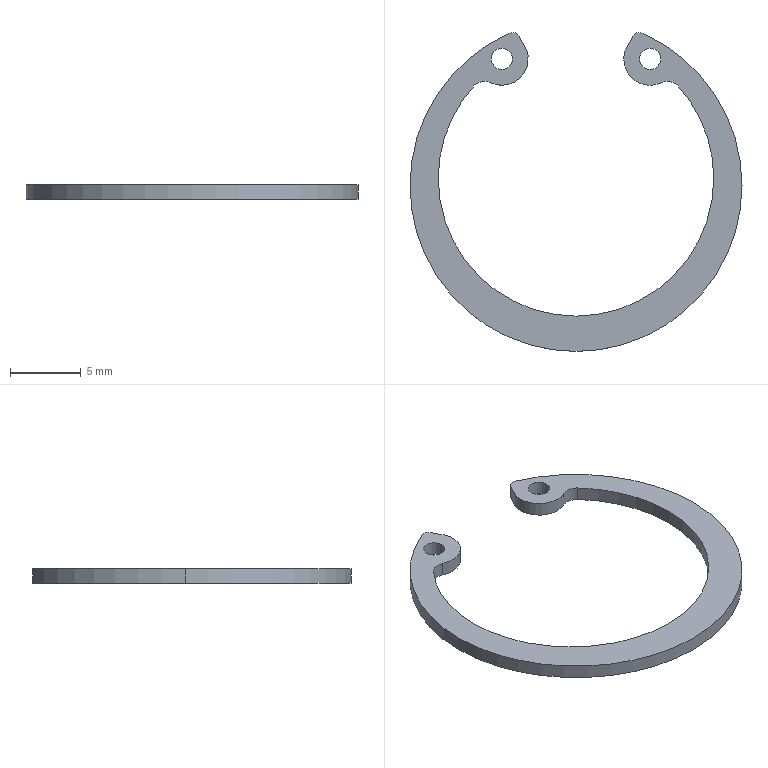Part | 1 solid | 21 faces | box 23.5 x 22.573 x 1 mm | volume 128.743 mm3 | cylinder 17 | plane 4 | commonest cylinder face diameters 1.5 x4 3.731 x3 19.5 x3 23.5 x3 1 x2 2 x2
STEP:
#1=CARTESIAN_POINT('',(4.5,8.954,1.));
#2=VERTEX_POINT('',#1);
#3=CARTESIAN_POINT('',(6.,8.954,1.));
#4=VERTEX_POINT('',#3);
#5=CARTESIAN_POINT('',(5.25,8.954,1.));
#6=DIRECTION('',(0.,0.,1.));
#7=DIRECTION('',(-1.,0.,0.));
#8=AXIS2_PLACEMENT_3D('',#5,#6,#7);
#9=CIRCLE('',#8,0.75);
#10=EDGE_CURVE('',#2,#4,#9,.T.);
#11=ORIENTED_EDGE('',*,*,#10,.T.);
#12=CARTESIAN_POINT('',(6.,8.954,0.));
#13=VERTEX_POINT('',#12);
#14=CARTESIAN_POINT('',(6.,8.954,1.));
#15=DIRECTION('',(0.,0.,-1.));
#16=VECTOR('',#15,1000.);
#17=LINE('',#14,#16);
#18=EDGE_CURVE('',#4,#13,#17,.T.);
#19=ORIENTED_EDGE('',*,*,#18,.T.);
#20=CARTESIAN_POINT('',(4.5,8.954,0.));
#21=VERTEX_POINT('',#20);
#22=CARTESIAN_POINT('',(5.25,8.954,0.));
#23=DIRECTION('',(0.,0.,1.));
#24=DIRECTION('',(-1.,0.,0.));
#25=AXIS2_PLACEMENT_3D('',#22,#23,#24);
#26=CIRCLE('',#25,0.75);
#27=EDGE_CURVE('',#21,#13,#26,.T.);
#28=ORIENTED_EDGE('',*,*,#27,.F.);
#29=CARTESIAN_POINT('',(4.5,8.954,1.));
#30=DIRECTION('',(0.,0.,-1.));
#31=VECTOR('',#30,1000.);
#32=LINE('',#29,#31);
#33=EDGE_CURVE('',#2,#21,#32,.T.);
#34=ORIENTED_EDGE('',*,*,#33,.F.);
#35=EDGE_LOOP('',(#11,#19,#28,#34));
#36=FACE_OUTER_BOUND('',#35,.T.);
#37=CARTESIAN_POINT('',(5.25,8.954,1.));
#38=DIRECTION('',(0.,0.,-1.));
#39=DIRECTION('',(-1.,0.,0.));
#40=AXIS2_PLACEMENT_3D('',#37,#38,#39);
#41=CYLINDRICAL_SURFACE('',#40,0.75);
#42=ADVANCED_FACE('',(#36),#41,.F.);
#43=CARTESIAN_POINT('',(-6.,8.954,1.));
#44=VERTEX_POINT('',#43);
#45=CARTESIAN_POINT('',(-4.5,8.954,1.));
#46=VERTEX_POINT('',#45);
#47=CARTESIAN_POINT('',(-5.25,8.954,1.));
#48=DIRECTION('',(0.,0.,1.));
#49=DIRECTION('',(1.,0.,0.));
#50=AXIS2_PLACEMENT_3D('',#47,#48,#49);
#51=CIRCLE('',#50,0.75);
#52=EDGE_CURVE('',#44,#46,#51,.T.);
#53=ORIENTED_EDGE('',*,*,#52,.T.);
#54=CARTESIAN_POINT('',(-4.5,8.954,0.));
#55=VERTEX_POINT('',#54);
#56=CARTESIAN_POINT('',(-4.5,8.954,1.));
#57=DIRECTION('',(0.,0.,-1.));
#58=VECTOR('',#57,1000.);
#59=LINE('',#56,#58);
#60=EDGE_CURVE('',#46,#55,#59,.T.);
#61=ORIENTED_EDGE('',*,*,#60,.T.);
#62=CARTESIAN_POINT('',(-6.,8.954,0.));
#63=VERTEX_POINT('',#62);
#64=CARTESIAN_POINT('',(-5.25,8.954,0.));
#65=DIRECTION('',(0.,0.,1.));
#66=DIRECTION('',(1.,0.,0.));
#67=AXIS2_PLACEMENT_3D('',#64,#65,#66);
#68=CIRCLE('',#67,0.75);
#69=EDGE_CURVE('',#63,#55,#68,.T.);
#70=ORIENTED_EDGE('',*,*,#69,.F.);
#71=CARTESIAN_POINT('',(-6.,8.954,1.));
#72=DIRECTION('',(0.,0.,-1.));
#73=VECTOR('',#72,1000.);
#74=LINE('',#71,#73);
#75=EDGE_CURVE('',#44,#63,#74,.T.);
#76=ORIENTED_EDGE('',*,*,#75,.F.);
#77=EDGE_LOOP('',(#53,#61,#70,#76));
#78=FACE_OUTER_BOUND('',#77,.T.);
#79=CARTESIAN_POINT('',(-5.25,8.954,1.));
#80=DIRECTION('',(0.,0.,-1.));
#81=DIRECTION('',(-1.,0.,0.));
#82=AXIS2_PLACEMENT_3D('',#79,#80,#81);
#83=CYLINDRICAL_SURFACE('',#82,0.75);
#84=ADVANCED_FACE('',(#78),#83,.F.);
#85=CARTESIAN_POINT('',(11.75,0.,1.));
#86=VERTEX_POINT('',#85);
#87=CARTESIAN_POINT('',(4.671,10.782,1.));
#88=VERTEX_POINT('',#87);
#89=CARTESIAN_POINT('',(0.,0.,1.));
#90=DIRECTION('',(0.,0.,1.));
#91=DIRECTION('',(1.,0.,0.));
#92=AXIS2_PLACEMENT_3D('',#89,#90,#91);
#93=CIRCLE('',#92,11.75);
#94=EDGE_CURVE('',#86,#88,#93,.T.);
#95=ORIENTED_EDGE('',*,*,#94,.F.);
#96=CARTESIAN_POINT('',(11.75,0.,0.));
#97=VERTEX_POINT('',#96);
#98=CARTESIAN_POINT('',(11.75,0.,1.));
#99=DIRECTION('',(0.,0.,-1.));
#100=VECTOR('',#99,1000.);
#101=LINE('',#98,#100);
#102=EDGE_CURVE('',#86,#97,#101,.T.);
#103=ORIENTED_EDGE('',*,*,#102,.T.);
#104=CARTESIAN_POINT('',(4.671,10.782,0.));
#105=VERTEX_POINT('',#104);
#106=CARTESIAN_POINT('',(0.,0.,0.));
#107=DIRECTION('',(0.,0.,1.));
#108=DIRECTION('',(1.,0.,0.));
#109=AXIS2_PLACEMENT_3D('',#106,#107,#108);
#110=CIRCLE('',#109,11.75);
#111=EDGE_CURVE('',#97,#105,#110,.T.);
#112=ORIENTED_EDGE('',*,*,#111,.T.);
#113=CARTESIAN_POINT('',(4.671,10.782,1.));
#114=DIRECTION('',(0.,0.,-1.));
#115=VECTOR('',#114,1000.);
#116=LINE('',#113,#115);
#117=EDGE_CURVE('',#88,#105,#116,.T.);
#118=ORIENTED_EDGE('',*,*,#117,.F.);
#119=EDGE_LOOP('',(#95,#103,#112,#118));
#120=FACE_OUTER_BOUND('',#119,.T.);
#121=CARTESIAN_POINT('',(0.,0.,1.));
#122=DIRECTION('',(0.,0.,-1.));
#123=DIRECTION('',(-1.,0.,0.));
#124=AXIS2_PLACEMENT_3D('',#121,#122,#123);
#125=CYLINDRICAL_SURFACE('',#124,11.75);
#126=ADVANCED_FACE('',(#120),#125,.T.);
#127=ORIENTED_EDGE('',*,*,#102,.F.);
#128=CARTESIAN_POINT('',(-11.75,0.,1.));
#129=VERTEX_POINT('',#128);
#130=CARTESIAN_POINT('',(0.,0.,1.));
#131=DIRECTION('',(0.,0.,1.));
#132=DIRECTION('',(1.,0.,0.));
#133=AXIS2_PLACEMENT_3D('',#130,#131,#132);
#134=CIRCLE('',#133,11.75);
#135=EDGE_CURVE('',#129,#86,#134,.T.);
#136=ORIENTED_EDGE('',*,*,#135,.F.);
#137=CARTESIAN_POINT('',(-11.75,0.,0.));
#138=VERTEX_POINT('',#137);
#139=CARTESIAN_POINT('',(-11.75,0.,1.));
#140=DIRECTION('',(0.,0.,-1.));
#141=VECTOR('',#140,1000.);
#142=LINE('',#139,#141);
#143=EDGE_CURVE('',#129,#138,#142,.T.);
#144=ORIENTED_EDGE('',*,*,#143,.T.);
#145=CARTESIAN_POINT('',(0.,0.,0.));
#146=DIRECTION('',(0.,0.,1.));
#147=DIRECTION('',(1.,0.,0.));
#148=AXIS2_PLACEMENT_3D('',#145,#146,#147);
#149=CIRCLE('',#148,11.75);
#150=EDGE_CURVE('',#138,#97,#149,.T.);
#151=ORIENTED_EDGE('',*,*,#150,.T.);
#152=EDGE_LOOP('',(#127,#136,#144,#151));
#153=FACE_OUTER_BOUND('',#152,.T.);
#154=CARTESIAN_POINT('',(0.,0.,1.));
#155=DIRECTION('',(0.,0.,-1.));
#156=DIRECTION('',(-1.,0.,0.));
#157=AXIS2_PLACEMENT_3D('',#154,#155,#156);
#158=CYLINDRICAL_SURFACE('',#157,11.75);
#159=ADVANCED_FACE('',(#153),#158,.T.);
#160=CARTESIAN_POINT('',(9.75,0.5,1.));
#161=VERTEX_POINT('',#160);
#162=CARTESIAN_POINT('',(-9.75,0.5,1.));
#163=VERTEX_POINT('',#162);
#164=CARTESIAN_POINT('',(0.,0.5,1.));
#165=DIRECTION('',(0.,0.,-1.));
#166=DIRECTION('',(1.,0.,0.));
#167=AXIS2_PLACEMENT_3D('',#164,#165,#166);
#168=CIRCLE('',#167,9.75);
#169=EDGE_CURVE('',#161,#163,#168,.T.);
#170=ORIENTED_EDGE('',*,*,#169,.F.);
#171=CARTESIAN_POINT('',(9.75,0.5,0.));
#172=VERTEX_POINT('',#171);
#173=CARTESIAN_POINT('',(9.75,0.5,1.));
#174=DIRECTION('',(0.,0.,-1.));
#175=VECTOR('',#174,1000.);
#176=LINE('',#173,#175);
#177=EDGE_CURVE('',#161,#172,#176,.T.);
#178=ORIENTED_EDGE('',*,*,#177,.T.);
#179=CARTESIAN_POINT('',(-9.75,0.5,0.));
#180=VERTEX_POINT('',#179);
#181=CARTESIAN_POINT('',(0.,0.5,0.));
#182=DIRECTION('',(0.,0.,-1.));
#183=DIRECTION('',(1.,0.,0.));
#184=AXIS2_PLACEMENT_3D('',#181,#182,#183);
#185=CIRCLE('',#184,9.75);
#186=EDGE_CURVE('',#172,#180,#185,.T.);
#187=ORIENTED_EDGE('',*,*,#186,.T.);
#188=CARTESIAN_POINT('',(-9.75,0.5,1.));
#189=DIRECTION('',(0.,0.,-1.));
#190=VECTOR('',#189,1000.);
#191=LINE('',#188,#190);
#192=EDGE_CURVE('',#163,#180,#191,.T.);
#193=ORIENTED_EDGE('',*,*,#192,.F.);
#194=EDGE_LOOP('',(#170,#178,#187,#193));
#195=FACE_OUTER_BOUND('',#194,.T.);
#196=CARTESIAN_POINT('',(0.,0.5,1.));
#197=DIRECTION('',(0.,0.,-1.));
#198=DIRECTION('',(-1.,0.,0.));
#199=AXIS2_PLACEMENT_3D('',#196,#197,#198);
#200=CYLINDRICAL_SURFACE('',#199,9.75);
#201=ADVANCED_FACE('',(#195),#200,.F.);
#202=CARTESIAN_POINT('',(-7.23,7.041,1.));
#203=VERTEX_POINT('',#202);
#204=CARTESIAN_POINT('',(0.,0.5,1.));
#205=DIRECTION('',(0.,0.,-1.));
#206=DIRECTION('',(1.,0.,0.));
#207=AXIS2_PLACEMENT_3D('',#204,#205,#206);
#208=CIRCLE('',#207,9.75);
#209=EDGE_CURVE('',#163,#203,#208,.T.);
#210=ORIENTED_EDGE('',*,*,#209,.F.);
#211=ORIENTED_EDGE('',*,*,#192,.T.);
#212=CARTESIAN_POINT('',(-7.23,7.041,0.));
#213=VERTEX_POINT('',#212);
#214=CARTESIAN_POINT('',(0.,0.5,0.));
#215=DIRECTION('',(0.,0.,-1.));
#216=DIRECTION('',(1.,0.,0.));
#217=AXIS2_PLACEMENT_3D('',#214,#215,#216);
#218=CIRCLE('',#217,9.75);
#219=EDGE_CURVE('',#180,#213,#218,.T.);
#220=ORIENTED_EDGE('',*,*,#219,.T.);
#221=CARTESIAN_POINT('',(-7.23,7.041,1.));
#222=DIRECTION('',(0.,0.,-1.));
#223=VECTOR('',#222,1000.);
#224=LINE('',#221,#223);
#225=EDGE_CURVE('',#203,#213,#224,.T.);
#226=ORIENTED_EDGE('',*,*,#225,.F.);
#227=EDGE_LOOP('',(#210,#211,#220,#226));
#228=FACE_OUTER_BOUND('',#227,.T.);
#229=CARTESIAN_POINT('',(0.,0.5,1.));
#230=DIRECTION('',(0.,0.,-1.));
#231=DIRECTION('',(-1.,0.,0.));
#232=AXIS2_PLACEMENT_3D('',#229,#230,#231);
#233=CYLINDRICAL_SURFACE('',#232,9.75);
#234=ADVANCED_FACE('',(#228),#233,.F.);
#235=CARTESIAN_POINT('',(3.385,8.954,1.));
#236=VERTEX_POINT('',#235);
#237=CARTESIAN_POINT('',(6.056,7.272,1.));
#238=VERTEX_POINT('',#237);
#239=CARTESIAN_POINT('',(5.25,8.954,1.));
#240=DIRECTION('',(0.,0.,1.));
#241=DIRECTION('',(-1.,0.,0.));
#242=AXIS2_PLACEMENT_3D('',#239,#240,#241);
#243=CIRCLE('',#242,1.865);
#244=EDGE_CURVE('',#236,#238,#243,.T.);
#245=ORIENTED_EDGE('',*,*,#244,.F.);
#246=CARTESIAN_POINT('',(3.385,8.954,0.));
#247=VERTEX_POINT('',#246);
#248=CARTESIAN_POINT('',(3.385,8.954,1.));
#249=DIRECTION('',(0.,0.,-1.));
#250=VECTOR('',#249,1000.);
#251=LINE('',#248,#250);
#252=EDGE_CURVE('',#236,#247,#251,.T.);
#253=ORIENTED_EDGE('',*,*,#252,.T.);
#254=CARTESIAN_POINT('',(6.056,7.272,0.));
#255=VERTEX_POINT('',#254);
#256=CARTESIAN_POINT('',(5.25,8.954,0.));
#257=DIRECTION('',(0.,0.,1.));
#258=DIRECTION('',(-1.,0.,0.));
#259=AXIS2_PLACEMENT_3D('',#256,#257,#258);
#260=CIRCLE('',#259,1.865);
#261=EDGE_CURVE('',#247,#255,#260,.T.);
#262=ORIENTED_EDGE('',*,*,#261,.T.);
#263=CARTESIAN_POINT('',(6.056,7.272,1.));
#264=DIRECTION('',(0.,0.,-1.));
#265=VECTOR('',#264,1000.);
#266=LINE('',#263,#265);
#267=EDGE_CURVE('',#238,#255,#266,.T.);
#268=ORIENTED_EDGE('',*,*,#267,.F.);
#269=EDGE_LOOP('',(#245,#253,#262,#268));
#270=FACE_OUTER_BOUND('',#269,.T.);
#271=CARTESIAN_POINT('',(5.25,8.954,1.));
#272=DIRECTION('',(0.,0.,-1.));
#273=DIRECTION('',(-1.,0.,0.));
#274=AXIS2_PLACEMENT_3D('',#271,#272,#273);
#275=CYLINDRICAL_SURFACE('',#274,1.865);
#276=ADVANCED_FACE('',(#270),#275,.T.);
#277=CARTESIAN_POINT('',(4.034,10.565,1.));
#278=VERTEX_POINT('',#277);
#279=CARTESIAN_POINT('',(4.472,10.323,1.));
#280=DIRECTION('',(0.,0.,1.));
#281=DIRECTION('',(-1.,0.,0.));
#282=AXIS2_PLACEMENT_3D('',#279,#280,#281);
#283=CIRCLE('',#282,0.5);
#284=EDGE_CURVE('',#88,#278,#283,.T.);
#285=ORIENTED_EDGE('',*,*,#284,.T.);
#286=CARTESIAN_POINT('',(3.5,9.6,1.));
#287=VERTEX_POINT('',#286);
#288=CARTESIAN_POINT('',(3.5,9.6,1.));
#289=DIRECTION('',(-0.4845,-0.8748,0.));
#290=VECTOR('',#289,1000.);
#291=LINE('',#288,#290);
#292=EDGE_CURVE('',#278,#287,#291,.T.);
#293=ORIENTED_EDGE('',*,*,#292,.T.);
#294=CARTESIAN_POINT('',(5.25,8.954,1.));
#295=DIRECTION('',(0.,0.,1.));
#296=DIRECTION('',(-1.,0.,0.));
#297=AXIS2_PLACEMENT_3D('',#294,#295,#296);
#298=CIRCLE('',#297,1.865);
#299=EDGE_CURVE('',#287,#236,#298,.T.);
#300=ORIENTED_EDGE('',*,*,#299,.T.);
#301=ORIENTED_EDGE('',*,*,#244,.T.);
#302=CARTESIAN_POINT('',(7.23,7.041,1.));
#303=VERTEX_POINT('',#302);
#304=CARTESIAN_POINT('',(6.488,6.371,1.));
#305=DIRECTION('',(0.,0.,-1.));
#306=DIRECTION('',(-1.,0.,0.));
#307=AXIS2_PLACEMENT_3D('',#304,#305,#306);
#308=CIRCLE('',#307,1.);
#309=EDGE_CURVE('',#238,#303,#308,.T.);
#310=ORIENTED_EDGE('',*,*,#309,.T.);
#311=CARTESIAN_POINT('',(0.,0.5,1.));
#312=DIRECTION('',(0.,0.,-1.));
#313=DIRECTION('',(1.,0.,0.));
#314=AXIS2_PLACEMENT_3D('',#311,#312,#313);
#315=CIRCLE('',#314,9.75);
#316=EDGE_CURVE('',#303,#161,#315,.T.);
#317=ORIENTED_EDGE('',*,*,#316,.T.);
#318=ORIENTED_EDGE('',*,*,#169,.T.);
#319=ORIENTED_EDGE('',*,*,#209,.T.);
#320=CARTESIAN_POINT('',(-6.056,7.272,1.));
#321=VERTEX_POINT('',#320);
#322=CARTESIAN_POINT('',(-6.488,6.371,1.));
#323=DIRECTION('',(0.,0.,-1.));
#324=DIRECTION('',(1.,0.,0.));
#325=AXIS2_PLACEMENT_3D('',#322,#323,#324);
#326=CIRCLE('',#325,1.);
#327=EDGE_CURVE('',#203,#321,#326,.T.);
#328=ORIENTED_EDGE('',*,*,#327,.T.);
#329=CARTESIAN_POINT('',(-3.5,9.6,1.));
#330=VERTEX_POINT('',#329);
#331=CARTESIAN_POINT('',(-5.25,8.954,1.));
#332=DIRECTION('',(0.,0.,1.));
#333=DIRECTION('',(1.,0.,0.));
#334=AXIS2_PLACEMENT_3D('',#331,#332,#333);
#335=CIRCLE('',#334,1.865);
#336=EDGE_CURVE('',#321,#330,#335,.T.);
#337=ORIENTED_EDGE('',*,*,#336,.T.);
#338=CARTESIAN_POINT('',(-4.034,10.565,1.));
#339=VERTEX_POINT('',#338);
#340=CARTESIAN_POINT('',(-3.5,9.6,1.));
#341=DIRECTION('',(-0.4845,0.8748,0.));
#342=VECTOR('',#341,1000.);
#343=LINE('',#340,#342);
#344=EDGE_CURVE('',#330,#339,#343,.T.);
#345=ORIENTED_EDGE('',*,*,#344,.T.);
#346=CARTESIAN_POINT('',(-4.671,10.782,1.));
#347=VERTEX_POINT('',#346);
#348=CARTESIAN_POINT('',(-4.472,10.323,1.));
#349=DIRECTION('',(0.,0.,1.));
#350=DIRECTION('',(1.,0.,0.));
#351=AXIS2_PLACEMENT_3D('',#348,#349,#350);
#352=CIRCLE('',#351,0.5);
#353=EDGE_CURVE('',#339,#347,#352,.T.);
#354=ORIENTED_EDGE('',*,*,#353,.T.);
#355=CARTESIAN_POINT('',(0.,0.,1.));
#356=DIRECTION('',(0.,0.,1.));
#357=DIRECTION('',(1.,0.,0.));
#358=AXIS2_PLACEMENT_3D('',#355,#356,#357);
#359=CIRCLE('',#358,11.75);
#360=EDGE_CURVE('',#347,#129,#359,.T.);
#361=ORIENTED_EDGE('',*,*,#360,.T.);
#362=ORIENTED_EDGE('',*,*,#135,.T.);
#363=ORIENTED_EDGE('',*,*,#94,.T.);
#364=EDGE_LOOP('',(#285,#293,#300,#301,#310,#317,#318,#319,#328,#337,#345,#354,#361,#362,#363));
#365=FACE_OUTER_BOUND('',#364,.T.);
#366=ORIENTED_EDGE('',*,*,#52,.F.);
#367=CARTESIAN_POINT('',(-5.25,8.954,1.));
#368=DIRECTION('',(0.,0.,1.));
#369=DIRECTION('',(1.,0.,0.));
#370=AXIS2_PLACEMENT_3D('',#367,#368,#369);
#371=CIRCLE('',#370,0.75);
#372=EDGE_CURVE('',#46,#44,#371,.T.);
#373=ORIENTED_EDGE('',*,*,#372,.F.);
#374=EDGE_LOOP('',(#366,#373));
#375=FACE_BOUND('',#374,.T.);
#376=ORIENTED_EDGE('',*,*,#10,.F.);
#377=CARTESIAN_POINT('',(5.25,8.954,1.));
#378=DIRECTION('',(0.,0.,1.));
#379=DIRECTION('',(-1.,0.,0.));
#380=AXIS2_PLACEMENT_3D('',#377,#378,#379);
#381=CIRCLE('',#380,0.75);
#382=EDGE_CURVE('',#4,#2,#381,.T.);
#383=ORIENTED_EDGE('',*,*,#382,.F.);
#384=EDGE_LOOP('',(#376,#383));
#385=FACE_BOUND('',#384,.T.);
#386=CARTESIAN_POINT('',(4.472,10.323,1.));
#387=DIRECTION('',(0.,0.,-1.));
#388=DIRECTION('',(0.,-1.,0.));
#389=AXIS2_PLACEMENT_3D('',#386,#387,#388);
#390=PLANE('',#389);
#391=ADVANCED_FACE('',(#365,#375,#385),#390,.F.);
#392=CARTESIAN_POINT('',(4.034,10.565,0.));
#393=VERTEX_POINT('',#392);
#394=CARTESIAN_POINT('',(4.472,10.323,0.));
#395=DIRECTION('',(0.,0.,1.));
#396=DIRECTION('',(-1.,0.,0.));
#397=AXIS2_PLACEMENT_3D('',#394,#395,#396);
#398=CIRCLE('',#397,0.5);
#399=EDGE_CURVE('',#105,#393,#398,.T.);
#400=ORIENTED_EDGE('',*,*,#399,.F.);
#401=ORIENTED_EDGE('',*,*,#111,.F.);
#402=ORIENTED_EDGE('',*,*,#150,.F.);
#403=CARTESIAN_POINT('',(-4.671,10.782,0.));
#404=VERTEX_POINT('',#403);
#405=CARTESIAN_POINT('',(0.,0.,0.));
#406=DIRECTION('',(0.,0.,1.));
#407=DIRECTION('',(1.,0.,0.));
#408=AXIS2_PLACEMENT_3D('',#405,#406,#407);
#409=CIRCLE('',#408,11.75);
#410=EDGE_CURVE('',#404,#138,#409,.T.);
#411=ORIENTED_EDGE('',*,*,#410,.F.);
#412=CARTESIAN_POINT('',(-4.034,10.565,0.));
#413=VERTEX_POINT('',#412);
#414=CARTESIAN_POINT('',(-4.472,10.323,0.));
#415=DIRECTION('',(0.,0.,1.));
#416=DIRECTION('',(1.,0.,0.));
#417=AXIS2_PLACEMENT_3D('',#414,#415,#416);
#418=CIRCLE('',#417,0.5);
#419=EDGE_CURVE('',#413,#404,#418,.T.);
#420=ORIENTED_EDGE('',*,*,#419,.F.);
#421=CARTESIAN_POINT('',(-3.5,9.6,0.));
#422=VERTEX_POINT('',#421);
#423=CARTESIAN_POINT('',(-3.5,9.6,0.));
#424=DIRECTION('',(-0.4845,0.8748,0.));
#425=VECTOR('',#424,1000.);
#426=LINE('',#423,#425);
#427=EDGE_CURVE('',#422,#413,#426,.T.);
#428=ORIENTED_EDGE('',*,*,#427,.F.);
#429=CARTESIAN_POINT('',(-6.056,7.272,0.));
#430=VERTEX_POINT('',#429);
#431=CARTESIAN_POINT('',(-5.25,8.954,0.));
#432=DIRECTION('',(0.,0.,1.));
#433=DIRECTION('',(1.,0.,0.));
#434=AXIS2_PLACEMENT_3D('',#431,#432,#433);
#435=CIRCLE('',#434,1.865);
#436=EDGE_CURVE('',#430,#422,#435,.T.);
#437=ORIENTED_EDGE('',*,*,#436,.F.);
#438=CARTESIAN_POINT('',(-6.488,6.371,0.));
#439=DIRECTION('',(0.,0.,-1.));
#440=DIRECTION('',(1.,0.,0.));
#441=AXIS2_PLACEMENT_3D('',#438,#439,#440);
#442=CIRCLE('',#441,1.);
#443=EDGE_CURVE('',#213,#430,#442,.T.);
#444=ORIENTED_EDGE('',*,*,#443,.F.);
#445=ORIENTED_EDGE('',*,*,#219,.F.);
#446=ORIENTED_EDGE('',*,*,#186,.F.);
#447=CARTESIAN_POINT('',(7.23,7.041,0.));
#448=VERTEX_POINT('',#447);
#449=CARTESIAN_POINT('',(0.,0.5,0.));
#450=DIRECTION('',(0.,0.,-1.));
#451=DIRECTION('',(1.,0.,0.));
#452=AXIS2_PLACEMENT_3D('',#449,#450,#451);
#453=CIRCLE('',#452,9.75);
#454=EDGE_CURVE('',#448,#172,#453,.T.);
#455=ORIENTED_EDGE('',*,*,#454,.F.);
#456=CARTESIAN_POINT('',(6.488,6.371,0.));
#457=DIRECTION('',(0.,0.,-1.));
#458=DIRECTION('',(-1.,0.,0.));
#459=AXIS2_PLACEMENT_3D('',#456,#457,#458);
#460=CIRCLE('',#459,1.);
#461=EDGE_CURVE('',#255,#448,#460,.T.);
#462=ORIENTED_EDGE('',*,*,#461,.F.);
#463=ORIENTED_EDGE('',*,*,#261,.F.);
#464=CARTESIAN_POINT('',(3.5,9.6,0.));
#465=VERTEX_POINT('',#464);
#466=CARTESIAN_POINT('',(5.25,8.954,0.));
#467=DIRECTION('',(0.,0.,1.));
#468=DIRECTION('',(-1.,0.,0.));
#469=AXIS2_PLACEMENT_3D('',#466,#467,#468);
#470=CIRCLE('',#469,1.865);
#471=EDGE_CURVE('',#465,#247,#470,.T.);
#472=ORIENTED_EDGE('',*,*,#471,.F.);
#473=CARTESIAN_POINT('',(3.5,9.6,0.));
#474=DIRECTION('',(-0.4845,-0.8748,0.));
#475=VECTOR('',#474,1000.);
#476=LINE('',#473,#475);
#477=EDGE_CURVE('',#393,#465,#476,.T.);
#478=ORIENTED_EDGE('',*,*,#477,.F.);
#479=EDGE_LOOP('',(#400,#401,#402,#411,#420,#428,#437,#444,#445,#446,#455,#462,#463,#472,#478));
#480=FACE_OUTER_BOUND('',#479,.T.);
#481=ORIENTED_EDGE('',*,*,#69,.T.);
#482=CARTESIAN_POINT('',(-5.25,8.954,0.));
#483=DIRECTION('',(0.,0.,1.));
#484=DIRECTION('',(1.,0.,0.));
#485=AXIS2_PLACEMENT_3D('',#482,#483,#484);
#486=CIRCLE('',#485,0.75);
#487=EDGE_CURVE('',#55,#63,#486,.T.);
#488=ORIENTED_EDGE('',*,*,#487,.T.);
#489=EDGE_LOOP('',(#481,#488));
#490=FACE_BOUND('',#489,.T.);
#491=ORIENTED_EDGE('',*,*,#27,.T.);
#492=CARTESIAN_POINT('',(5.25,8.954,0.));
#493=DIRECTION('',(0.,0.,1.));
#494=DIRECTION('',(-1.,0.,0.));
#495=AXIS2_PLACEMENT_3D('',#492,#493,#494);
#496=CIRCLE('',#495,0.75);
#497=EDGE_CURVE('',#13,#21,#496,.T.);
#498=ORIENTED_EDGE('',*,*,#497,.T.);
#499=EDGE_LOOP('',(#491,#498));
#500=FACE_BOUND('',#499,.T.);
#501=CARTESIAN_POINT('',(4.472,10.323,0.));
#502=DIRECTION('',(0.,0.,-1.));
#503=DIRECTION('',(0.,-1.,0.));
#504=AXIS2_PLACEMENT_3D('',#501,#502,#503);
#505=PLANE('',#504);
#506=ADVANCED_FACE('',(#480,#490,#500),#505,.T.);
#507=ORIENTED_EDGE('',*,*,#399,.T.);
#508=CARTESIAN_POINT('',(4.034,10.565,1.));
#509=DIRECTION('',(0.,0.,-1.));
#510=VECTOR('',#509,1000.);
#511=LINE('',#508,#510);
#512=EDGE_CURVE('',#278,#393,#511,.T.);
#513=ORIENTED_EDGE('',*,*,#512,.F.);
#514=ORIENTED_EDGE('',*,*,#284,.F.);
#515=ORIENTED_EDGE('',*,*,#117,.T.);
#516=EDGE_LOOP('',(#507,#513,#514,#515));
#517=FACE_OUTER_BOUND('',#516,.T.);
#518=CARTESIAN_POINT('',(4.472,10.323,1.));
#519=DIRECTION('',(0.,0.,-1.));
#520=DIRECTION('',(-1.,0.,0.));
#521=AXIS2_PLACEMENT_3D('',#518,#519,#520);
#522=CYLINDRICAL_SURFACE('',#521,0.5);
#523=ADVANCED_FACE('',(#517),#522,.T.);
#524=ORIENTED_EDGE('',*,*,#477,.T.);
#525=CARTESIAN_POINT('',(3.5,9.6,1.));
#526=DIRECTION('',(0.,0.,-1.));
#527=VECTOR('',#526,1000.);
#528=LINE('',#525,#527);
#529=EDGE_CURVE('',#287,#465,#528,.T.);
#530=ORIENTED_EDGE('',*,*,#529,.F.);
#531=ORIENTED_EDGE('',*,*,#292,.F.);
#532=ORIENTED_EDGE('',*,*,#512,.T.);
#533=EDGE_LOOP('',(#524,#530,#531,#532));
#534=FACE_OUTER_BOUND('',#533,.T.);
#535=CARTESIAN_POINT('',(3.5,9.6,1.));
#536=DIRECTION('',(0.8748,-0.4845,0.));
#537=DIRECTION('',(0.,0.,-1.));
#538=AXIS2_PLACEMENT_3D('',#535,#536,#537);
#539=PLANE('',#538);
#540=ADVANCED_FACE('',(#534),#539,.F.);
#541=ORIENTED_EDGE('',*,*,#252,.F.);
#542=ORIENTED_EDGE('',*,*,#299,.F.);
#543=ORIENTED_EDGE('',*,*,#529,.T.);
#544=ORIENTED_EDGE('',*,*,#471,.T.);
#545=EDGE_LOOP('',(#541,#542,#543,#544));
#546=FACE_OUTER_BOUND('',#545,.T.);
#547=CARTESIAN_POINT('',(5.25,8.954,1.));
#548=DIRECTION('',(0.,0.,-1.));
#549=DIRECTION('',(-1.,0.,0.));
#550=AXIS2_PLACEMENT_3D('',#547,#548,#549);
#551=CYLINDRICAL_SURFACE('',#550,1.865);
#552=ADVANCED_FACE('',(#546),#551,.T.);
#553=ORIENTED_EDGE('',*,*,#461,.T.);
#554=CARTESIAN_POINT('',(7.23,7.041,1.));
#555=DIRECTION('',(0.,0.,-1.));
#556=VECTOR('',#555,1000.);
#557=LINE('',#554,#556);
#558=EDGE_CURVE('',#303,#448,#557,.T.);
#559=ORIENTED_EDGE('',*,*,#558,.F.);
#560=ORIENTED_EDGE('',*,*,#309,.F.);
#561=ORIENTED_EDGE('',*,*,#267,.T.);
#562=EDGE_LOOP('',(#553,#559,#560,#561));
#563=FACE_OUTER_BOUND('',#562,.T.);
#564=CARTESIAN_POINT('',(6.488,6.371,1.));
#565=DIRECTION('',(0.,0.,-1.));
#566=DIRECTION('',(-1.,0.,0.));
#567=AXIS2_PLACEMENT_3D('',#564,#565,#566);
#568=CYLINDRICAL_SURFACE('',#567,1.);
#569=ADVANCED_FACE('',(#563),#568,.F.);
#570=ORIENTED_EDGE('',*,*,#177,.F.);
#571=ORIENTED_EDGE('',*,*,#316,.F.);
#572=ORIENTED_EDGE('',*,*,#558,.T.);
#573=ORIENTED_EDGE('',*,*,#454,.T.);
#574=EDGE_LOOP('',(#570,#571,#572,#573));
#575=FACE_OUTER_BOUND('',#574,.T.);
#576=CARTESIAN_POINT('',(0.,0.5,1.));
#577=DIRECTION('',(0.,0.,-1.));
#578=DIRECTION('',(-1.,0.,0.));
#579=AXIS2_PLACEMENT_3D('',#576,#577,#578);
#580=CYLINDRICAL_SURFACE('',#579,9.75);
#581=ADVANCED_FACE('',(#575),#580,.F.);
#582=ORIENTED_EDGE('',*,*,#443,.T.);
#583=CARTESIAN_POINT('',(-6.056,7.272,1.));
#584=DIRECTION('',(0.,0.,-1.));
#585=VECTOR('',#584,1000.);
#586=LINE('',#583,#585);
#587=EDGE_CURVE('',#321,#430,#586,.T.);
#588=ORIENTED_EDGE('',*,*,#587,.F.);
#589=ORIENTED_EDGE('',*,*,#327,.F.);
#590=ORIENTED_EDGE('',*,*,#225,.T.);
#591=EDGE_LOOP('',(#582,#588,#589,#590));
#592=FACE_OUTER_BOUND('',#591,.T.);
#593=CARTESIAN_POINT('',(-6.488,6.371,1.));
#594=DIRECTION('',(0.,0.,-1.));
#595=DIRECTION('',(-1.,0.,0.));
#596=AXIS2_PLACEMENT_3D('',#593,#594,#595);
#597=CYLINDRICAL_SURFACE('',#596,1.);
#598=ADVANCED_FACE('',(#592),#597,.F.);
#599=ORIENTED_EDGE('',*,*,#436,.T.);
#600=CARTESIAN_POINT('',(-3.5,9.6,1.));
#601=DIRECTION('',(0.,0.,-1.));
#602=VECTOR('',#601,1000.);
#603=LINE('',#600,#602);
#604=EDGE_CURVE('',#330,#422,#603,.T.);
#605=ORIENTED_EDGE('',*,*,#604,.F.);
#606=ORIENTED_EDGE('',*,*,#336,.F.);
#607=ORIENTED_EDGE('',*,*,#587,.T.);
#608=EDGE_LOOP('',(#599,#605,#606,#607));
#609=FACE_OUTER_BOUND('',#608,.T.);
#610=CARTESIAN_POINT('',(-5.25,8.954,1.));
#611=DIRECTION('',(0.,0.,-1.));
#612=DIRECTION('',(-1.,0.,0.));
#613=AXIS2_PLACEMENT_3D('',#610,#611,#612);
#614=CYLINDRICAL_SURFACE('',#613,1.865);
#615=ADVANCED_FACE('',(#609),#614,.T.);
#616=ORIENTED_EDGE('',*,*,#427,.T.);
#617=CARTESIAN_POINT('',(-4.034,10.565,1.));
#618=DIRECTION('',(0.,0.,-1.));
#619=VECTOR('',#618,1000.);
#620=LINE('',#617,#619);
#621=EDGE_CURVE('',#339,#413,#620,.T.);
#622=ORIENTED_EDGE('',*,*,#621,.F.);
#623=ORIENTED_EDGE('',*,*,#344,.F.);
#624=ORIENTED_EDGE('',*,*,#604,.T.);
#625=EDGE_LOOP('',(#616,#622,#623,#624));
#626=FACE_OUTER_BOUND('',#625,.T.);
#627=CARTESIAN_POINT('',(-3.5,9.6,1.));
#628=DIRECTION('',(-0.8748,-0.4845,0.));
#629=DIRECTION('',(-0.4845,0.8748,0.));
#630=AXIS2_PLACEMENT_3D('',#627,#628,#629);
#631=PLANE('',#630);
#632=ADVANCED_FACE('',(#626),#631,.F.);
#633=ORIENTED_EDGE('',*,*,#419,.T.);
#634=CARTESIAN_POINT('',(-4.671,10.782,1.));
#635=DIRECTION('',(0.,0.,-1.));
#636=VECTOR('',#635,1000.);
#637=LINE('',#634,#636);
#638=EDGE_CURVE('',#347,#404,#637,.T.);
#639=ORIENTED_EDGE('',*,*,#638,.F.);
#640=ORIENTED_EDGE('',*,*,#353,.F.);
#641=ORIENTED_EDGE('',*,*,#621,.T.);
#642=EDGE_LOOP('',(#633,#639,#640,#641));
#643=FACE_OUTER_BOUND('',#642,.T.);
#644=CARTESIAN_POINT('',(-4.472,10.323,1.));
#645=DIRECTION('',(0.,0.,-1.));
#646=DIRECTION('',(-1.,0.,0.));
#647=AXIS2_PLACEMENT_3D('',#644,#645,#646);
#648=CYLINDRICAL_SURFACE('',#647,0.5);
#649=ADVANCED_FACE('',(#643),#648,.T.);
#650=ORIENTED_EDGE('',*,*,#143,.F.);
#651=ORIENTED_EDGE('',*,*,#360,.F.);
#652=ORIENTED_EDGE('',*,*,#638,.T.);
#653=ORIENTED_EDGE('',*,*,#410,.T.);
#654=EDGE_LOOP('',(#650,#651,#652,#653));
#655=FACE_OUTER_BOUND('',#654,.T.);
#656=CARTESIAN_POINT('',(0.,0.,1.));
#657=DIRECTION('',(0.,0.,-1.));
#658=DIRECTION('',(-1.,0.,0.));
#659=AXIS2_PLACEMENT_3D('',#656,#657,#658);
#660=CYLINDRICAL_SURFACE('',#659,11.75);
#661=ADVANCED_FACE('',(#655),#660,.T.);
#662=ORIENTED_EDGE('',*,*,#60,.F.);
#663=ORIENTED_EDGE('',*,*,#372,.T.);
#664=ORIENTED_EDGE('',*,*,#75,.T.);
#665=ORIENTED_EDGE('',*,*,#487,.F.);
#666=EDGE_LOOP('',(#662,#663,#664,#665));
#667=FACE_OUTER_BOUND('',#666,.T.);
#668=CARTESIAN_POINT('',(-5.25,8.954,1.));
#669=DIRECTION('',(0.,0.,-1.));
#670=DIRECTION('',(-1.,0.,0.));
#671=AXIS2_PLACEMENT_3D('',#668,#669,#670);
#672=CYLINDRICAL_SURFACE('',#671,0.75);
#673=ADVANCED_FACE('',(#667),#672,.F.);
#674=ORIENTED_EDGE('',*,*,#18,.F.);
#675=ORIENTED_EDGE('',*,*,#382,.T.);
#676=ORIENTED_EDGE('',*,*,#33,.T.);
#677=ORIENTED_EDGE('',*,*,#497,.F.);
#678=EDGE_LOOP('',(#674,#675,#676,#677));
#679=FACE_OUTER_BOUND('',#678,.T.);
#680=CARTESIAN_POINT('',(5.25,8.954,1.));
#681=DIRECTION('',(0.,0.,-1.));
#682=DIRECTION('',(-1.,0.,0.));
#683=AXIS2_PLACEMENT_3D('',#680,#681,#682);
#684=CYLINDRICAL_SURFACE('',#683,0.75);
#685=ADVANCED_FACE('',(#679),#684,.F.);
#686=CLOSED_SHELL('',(#42,#84,#126,#159,#201,#234,#276,#391,#506,#523,#540,#552,#569,#581,#598,#615,#632,#649,#661,#673,#685));
#687=MANIFOLD_SOLID_BREP('',#686);
#688=CARTESIAN_POINT('',(0.,0.,0.));
#689=DIRECTION('',(0.,0.,1.));
#690=DIRECTION('',(1.,0.,0.));
#691=AXIS2_PLACEMENT_3D('',#688,#689,#690);
#692=(LENGTH_UNIT()NAMED_UNIT(*)SI_UNIT(.MILLI.,.METRE.));
#693=UNCERTAINTY_MEASURE_WITH_UNIT(LENGTH_MEASURE(0.00001),#692,'','');
#694=(NAMED_UNIT(*)PLANE_ANGLE_UNIT()SI_UNIT($,.RADIAN.));
#695=(NAMED_UNIT(*)SI_UNIT($,.STERADIAN.)SOLID_ANGLE_UNIT());
#696=(GEOMETRIC_REPRESENTATION_CONTEXT(3)GLOBAL_UNCERTAINTY_ASSIGNED_CONTEXT((#693))GLOBAL_UNIT_ASSIGNED_CONTEXT((#692,#694,#695))REPRESENTATION_CONTEXT('',''));
#697=ADVANCED_BREP_SHAPE_REPRESENTATION('',(#687,#691),#696);